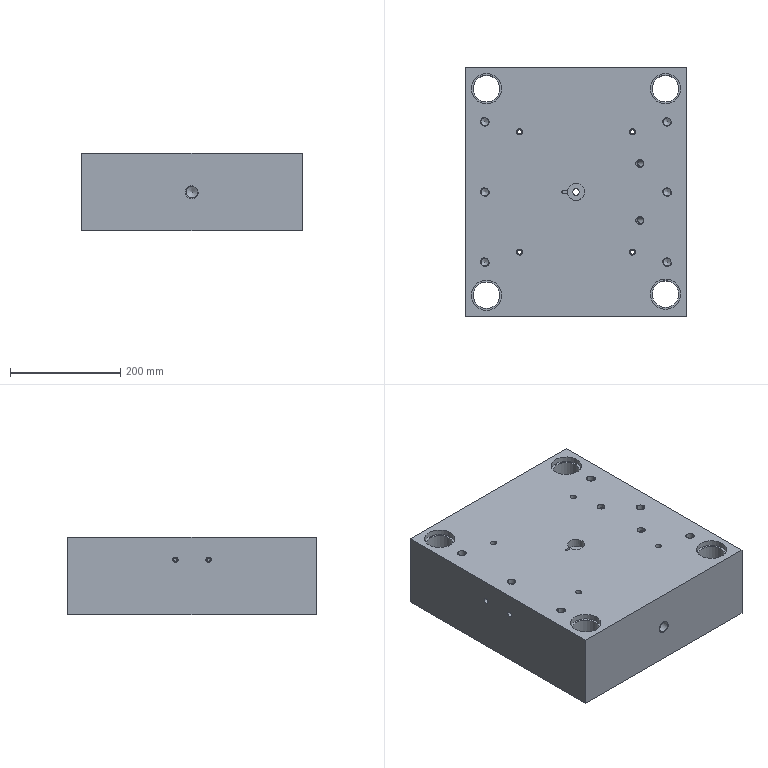Part | NX | features solid 2 | 1 solid | 162 faces | box 400 x 450 x 140 mm | volume 19391135 mm3 | plane 83 | cylinder 63 | cone 16 | commonest cylinder face diameters 11 x6 14.1 x6 15.7 x6 16 x6 6 x4 7 x4